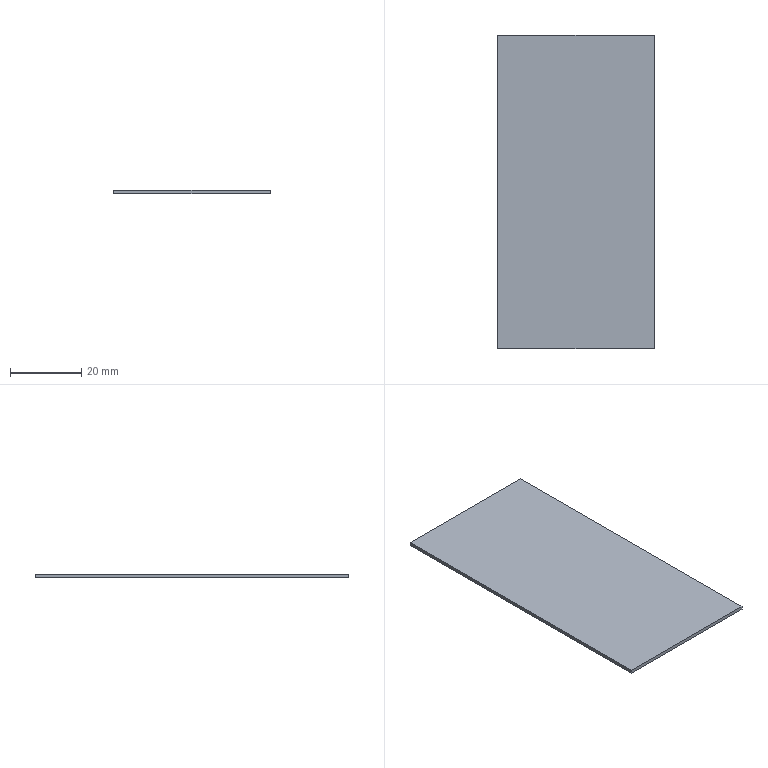Part | 1 solid | 6 faces | box 44 x 88 x 1 mm | volume 3872 mm3 | plane 6
STEP:
#1=CARTESIAN_POINT('',(22.,-44.,-0.5));
#2=VERTEX_POINT('',#1);
#3=CARTESIAN_POINT('',(22.,44.,-0.5));
#4=VERTEX_POINT('',#3);
#5=CARTESIAN_POINT('',(22.,-44.,-0.5));
#6=DIRECTION('',(0.,1.,0.));
#7=VECTOR('',#6,1000.);
#8=LINE('',#5,#7);
#9=EDGE_CURVE('',#2,#4,#8,.T.);
#10=ORIENTED_EDGE('',*,*,#9,.T.);
#11=CARTESIAN_POINT('',(22.,44.,0.5));
#12=VERTEX_POINT('',#11);
#13=CARTESIAN_POINT('',(22.,44.,0.5));
#14=DIRECTION('',(0.,0.,-1.));
#15=VECTOR('',#14,1000.);
#16=LINE('',#13,#15);
#17=EDGE_CURVE('',#12,#4,#16,.T.);
#18=ORIENTED_EDGE('',*,*,#17,.F.);
#19=CARTESIAN_POINT('',(22.,-44.,0.5));
#20=VERTEX_POINT('',#19);
#21=CARTESIAN_POINT('',(22.,-44.,0.5));
#22=DIRECTION('',(0.,1.,0.));
#23=VECTOR('',#22,1000.);
#24=LINE('',#21,#23);
#25=EDGE_CURVE('',#20,#12,#24,.T.);
#26=ORIENTED_EDGE('',*,*,#25,.F.);
#27=CARTESIAN_POINT('',(22.,-44.,0.5));
#28=DIRECTION('',(0.,0.,-1.));
#29=VECTOR('',#28,1000.);
#30=LINE('',#27,#29);
#31=EDGE_CURVE('',#20,#2,#30,.T.);
#32=ORIENTED_EDGE('',*,*,#31,.T.);
#33=EDGE_LOOP('',(#10,#18,#26,#32));
#34=FACE_OUTER_BOUND('',#33,.T.);
#35=CARTESIAN_POINT('',(22.,-44.,0.5));
#36=DIRECTION('',(-1.,0.,0.));
#37=DIRECTION('',(0.,0.,1.));
#38=AXIS2_PLACEMENT_3D('',#35,#36,#37);
#39=PLANE('',#38);
#40=ADVANCED_FACE('',(#34),#39,.F.);
#41=CARTESIAN_POINT('',(-22.,44.,-0.5));
#42=VERTEX_POINT('',#41);
#43=CARTESIAN_POINT('',(-22.,44.,-0.5));
#44=DIRECTION('',(-1.,0.,0.));
#45=VECTOR('',#44,1000.);
#46=LINE('',#43,#45);
#47=EDGE_CURVE('',#4,#42,#46,.T.);
#48=ORIENTED_EDGE('',*,*,#47,.T.);
#49=CARTESIAN_POINT('',(-22.,44.,0.5));
#50=VERTEX_POINT('',#49);
#51=CARTESIAN_POINT('',(-22.,44.,0.5));
#52=DIRECTION('',(0.,0.,-1.));
#53=VECTOR('',#52,1000.);
#54=LINE('',#51,#53);
#55=EDGE_CURVE('',#50,#42,#54,.T.);
#56=ORIENTED_EDGE('',*,*,#55,.F.);
#57=CARTESIAN_POINT('',(-22.,44.,0.5));
#58=DIRECTION('',(-1.,0.,0.));
#59=VECTOR('',#58,1000.);
#60=LINE('',#57,#59);
#61=EDGE_CURVE('',#12,#50,#60,.T.);
#62=ORIENTED_EDGE('',*,*,#61,.F.);
#63=ORIENTED_EDGE('',*,*,#17,.T.);
#64=EDGE_LOOP('',(#48,#56,#62,#63));
#65=FACE_OUTER_BOUND('',#64,.T.);
#66=CARTESIAN_POINT('',(-22.,44.,0.5));
#67=DIRECTION('',(0.,-1.,0.));
#68=DIRECTION('',(0.,0.,-1.));
#69=AXIS2_PLACEMENT_3D('',#66,#67,#68);
#70=PLANE('',#69);
#71=ADVANCED_FACE('',(#65),#70,.F.);
#72=CARTESIAN_POINT('',(-22.,-44.,-0.5));
#73=VERTEX_POINT('',#72);
#74=CARTESIAN_POINT('',(-22.,-44.,-0.5));
#75=DIRECTION('',(0.,-1.,0.));
#76=VECTOR('',#75,1000.);
#77=LINE('',#74,#76);
#78=EDGE_CURVE('',#42,#73,#77,.T.);
#79=ORIENTED_EDGE('',*,*,#78,.T.);
#80=CARTESIAN_POINT('',(-22.,-44.,0.5));
#81=VERTEX_POINT('',#80);
#82=CARTESIAN_POINT('',(-22.,-44.,0.5));
#83=DIRECTION('',(0.,0.,-1.));
#84=VECTOR('',#83,1000.);
#85=LINE('',#82,#84);
#86=EDGE_CURVE('',#81,#73,#85,.T.);
#87=ORIENTED_EDGE('',*,*,#86,.F.);
#88=CARTESIAN_POINT('',(-22.,-44.,0.5));
#89=DIRECTION('',(0.,-1.,0.));
#90=VECTOR('',#89,1000.);
#91=LINE('',#88,#90);
#92=EDGE_CURVE('',#50,#81,#91,.T.);
#93=ORIENTED_EDGE('',*,*,#92,.F.);
#94=ORIENTED_EDGE('',*,*,#55,.T.);
#95=EDGE_LOOP('',(#79,#87,#93,#94));
#96=FACE_OUTER_BOUND('',#95,.T.);
#97=CARTESIAN_POINT('',(-22.,-44.,0.5));
#98=DIRECTION('',(1.,0.,0.));
#99=DIRECTION('',(0.,0.,-1.));
#100=AXIS2_PLACEMENT_3D('',#97,#98,#99);
#101=PLANE('',#100);
#102=ADVANCED_FACE('',(#96),#101,.F.);
#103=CARTESIAN_POINT('',(-22.,-44.,-0.5));
#104=DIRECTION('',(1.,0.,0.));
#105=VECTOR('',#104,1000.);
#106=LINE('',#103,#105);
#107=EDGE_CURVE('',#73,#2,#106,.T.);
#108=ORIENTED_EDGE('',*,*,#107,.T.);
#109=ORIENTED_EDGE('',*,*,#31,.F.);
#110=CARTESIAN_POINT('',(-22.,-44.,0.5));
#111=DIRECTION('',(1.,0.,0.));
#112=VECTOR('',#111,1000.);
#113=LINE('',#110,#112);
#114=EDGE_CURVE('',#81,#20,#113,.T.);
#115=ORIENTED_EDGE('',*,*,#114,.F.);
#116=ORIENTED_EDGE('',*,*,#86,.T.);
#117=EDGE_LOOP('',(#108,#109,#115,#116));
#118=FACE_OUTER_BOUND('',#117,.T.);
#119=CARTESIAN_POINT('',(-22.,-44.,0.5));
#120=DIRECTION('',(0.,1.,0.));
#121=DIRECTION('',(0.,0.,1.));
#122=AXIS2_PLACEMENT_3D('',#119,#120,#121);
#123=PLANE('',#122);
#124=ADVANCED_FACE('',(#118),#123,.F.);
#125=ORIENTED_EDGE('',*,*,#25,.T.);
#126=ORIENTED_EDGE('',*,*,#61,.T.);
#127=ORIENTED_EDGE('',*,*,#92,.T.);
#128=ORIENTED_EDGE('',*,*,#114,.T.);
#129=EDGE_LOOP('',(#125,#126,#127,#128));
#130=FACE_OUTER_BOUND('',#129,.T.);
#131=CARTESIAN_POINT('',(0.,0.,0.5));
#132=DIRECTION('',(0.,0.,-1.));
#133=DIRECTION('',(-1.,0.,0.));
#134=AXIS2_PLACEMENT_3D('',#131,#132,#133);
#135=PLANE('',#134);
#136=ADVANCED_FACE('',(#130),#135,.F.);
#137=ORIENTED_EDGE('',*,*,#9,.F.);
#138=ORIENTED_EDGE('',*,*,#107,.F.);
#139=ORIENTED_EDGE('',*,*,#78,.F.);
#140=ORIENTED_EDGE('',*,*,#47,.F.);
#141=EDGE_LOOP('',(#137,#138,#139,#140));
#142=FACE_OUTER_BOUND('',#141,.T.);
#143=CARTESIAN_POINT('',(0.,0.,-0.5));
#144=DIRECTION('',(0.,0.,-1.));
#145=DIRECTION('',(-1.,0.,0.));
#146=AXIS2_PLACEMENT_3D('',#143,#144,#145);
#147=PLANE('',#146);
#148=ADVANCED_FACE('',(#142),#147,.T.);
#149=CLOSED_SHELL('',(#40,#71,#102,#124,#136,#148));
#150=MANIFOLD_SOLID_BREP('',#149);
#151=CARTESIAN_POINT('',(0.,0.,0.));
#152=DIRECTION('',(0.,0.,1.));
#153=DIRECTION('',(1.,0.,0.));
#154=AXIS2_PLACEMENT_3D('',#151,#152,#153);
#155=(LENGTH_UNIT()NAMED_UNIT(*)SI_UNIT(.MILLI.,.METRE.));
#156=UNCERTAINTY_MEASURE_WITH_UNIT(LENGTH_MEASURE(0.00001),#155,'','');
#157=(NAMED_UNIT(*)PLANE_ANGLE_UNIT()SI_UNIT($,.RADIAN.));
#158=(NAMED_UNIT(*)SI_UNIT($,.STERADIAN.)SOLID_ANGLE_UNIT());
#159=(GEOMETRIC_REPRESENTATION_CONTEXT(3)GLOBAL_UNCERTAINTY_ASSIGNED_CONTEXT((#156))GLOBAL_UNIT_ASSIGNED_CONTEXT((#155,#157,#158))REPRESENTATION_CONTEXT('',''));
#160=ADVANCED_BREP_SHAPE_REPRESENTATION('',(#150,#154),#159);